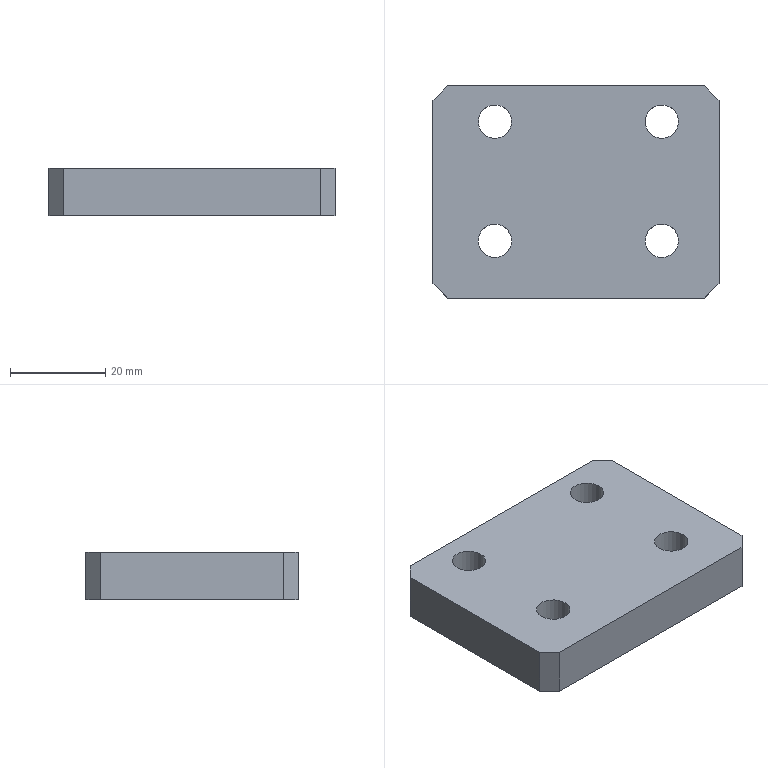Part | NX | features BREP 1 | 1 solid | 14 faces | box 60 x 44.5 x 10 mm | volume 24981 mm3 | plane 10 | cylinder 4 | commonest cylinder face diameters 7 x4
STEP:
#1=CARTESIAN_POINT('',(30.,-19.25,0.));
#2=VERTEX_POINT('',#1);
#3=CARTESIAN_POINT('',(30.,19.25,0.));
#4=VERTEX_POINT('',#3);
#5=CARTESIAN_POINT('',(30.,22.25,0.));
#6=DIRECTION('',(0.,1.,0.));
#7=VECTOR('',#6,1000.);
#8=LINE('',#5,#7);
#9=EDGE_CURVE('',#2,#4,#8,.T.);
#10=ORIENTED_EDGE('',*,*,#9,.T.);
#11=CARTESIAN_POINT('',(30.,19.25,10.));
#12=VERTEX_POINT('',#11);
#13=CARTESIAN_POINT('',(30.,19.25,10.));
#14=DIRECTION('',(0.,0.,1.));
#15=VECTOR('',#14,1000.);
#16=LINE('',#13,#15);
#17=EDGE_CURVE('',#4,#12,#16,.T.);
#18=ORIENTED_EDGE('',*,*,#17,.T.);
#19=CARTESIAN_POINT('',(30.,-19.25,10.));
#20=VERTEX_POINT('',#19);
#21=CARTESIAN_POINT('',(30.,22.25,10.));
#22=DIRECTION('',(0.,1.,0.));
#23=VECTOR('',#22,1000.);
#24=LINE('',#21,#23);
#25=EDGE_CURVE('',#20,#12,#24,.T.);
#26=ORIENTED_EDGE('',*,*,#25,.F.);
#27=CARTESIAN_POINT('',(30.,-19.25,10.));
#28=DIRECTION('',(0.,0.,-1.));
#29=VECTOR('',#28,1000.);
#30=LINE('',#27,#29);
#31=EDGE_CURVE('',#20,#2,#30,.T.);
#32=ORIENTED_EDGE('',*,*,#31,.T.);
#33=EDGE_LOOP('',(#10,#18,#26,#32));
#34=FACE_BOUND('',#33,.T.);
#35=CARTESIAN_POINT('',(30.,22.25,10.));
#36=DIRECTION('',(-1.,0.,0.));
#37=DIRECTION('',(0.,1.,0.));
#38=AXIS2_PLACEMENT_3D('',#35,#36,#37);
#39=PLANE('',#38);
#40=ADVANCED_FACE('',(#34),#39,.F.);
#41=CARTESIAN_POINT('',(27.,22.25,10.));
#42=VERTEX_POINT('',#41);
#43=CARTESIAN_POINT('',(-27.,22.25,10.));
#44=VERTEX_POINT('',#43);
#45=CARTESIAN_POINT('',(-30.,22.25,10.));
#46=DIRECTION('',(-1.,0.,0.));
#47=VECTOR('',#46,1000.);
#48=LINE('',#45,#47);
#49=EDGE_CURVE('',#42,#44,#48,.T.);
#50=ORIENTED_EDGE('',*,*,#49,.F.);
#51=CARTESIAN_POINT('',(27.,22.25,0.));
#52=VERTEX_POINT('',#51);
#53=CARTESIAN_POINT('',(27.,22.25,10.));
#54=DIRECTION('',(0.,0.,-1.));
#55=VECTOR('',#54,1000.);
#56=LINE('',#53,#55);
#57=EDGE_CURVE('',#42,#52,#56,.T.);
#58=ORIENTED_EDGE('',*,*,#57,.T.);
#59=CARTESIAN_POINT('',(-27.,22.25,0.));
#60=VERTEX_POINT('',#59);
#61=CARTESIAN_POINT('',(-30.,22.25,0.));
#62=DIRECTION('',(-1.,0.,0.));
#63=VECTOR('',#62,1000.);
#64=LINE('',#61,#63);
#65=EDGE_CURVE('',#52,#60,#64,.T.);
#66=ORIENTED_EDGE('',*,*,#65,.T.);
#67=CARTESIAN_POINT('',(-27.,22.25,10.));
#68=DIRECTION('',(0.,0.,1.));
#69=VECTOR('',#68,1000.);
#70=LINE('',#67,#69);
#71=EDGE_CURVE('',#60,#44,#70,.T.);
#72=ORIENTED_EDGE('',*,*,#71,.T.);
#73=EDGE_LOOP('',(#50,#58,#66,#72));
#74=FACE_BOUND('',#73,.T.);
#75=CARTESIAN_POINT('',(-30.,22.25,10.));
#76=DIRECTION('',(0.,-1.,0.));
#77=DIRECTION('',(0.,0.,1.));
#78=AXIS2_PLACEMENT_3D('',#75,#76,#77);
#79=PLANE('',#78);
#80=ADVANCED_FACE('',(#74),#79,.F.);
#81=CARTESIAN_POINT('',(-30.,19.25,10.));
#82=VERTEX_POINT('',#81);
#83=CARTESIAN_POINT('',(-30.,-19.25,10.));
#84=VERTEX_POINT('',#83);
#85=CARTESIAN_POINT('',(-30.,22.25,10.));
#86=DIRECTION('',(0.,-1.,0.));
#87=VECTOR('',#86,1000.);
#88=LINE('',#85,#87);
#89=EDGE_CURVE('',#82,#84,#88,.T.);
#90=ORIENTED_EDGE('',*,*,#89,.F.);
#91=CARTESIAN_POINT('',(-30.,19.25,0.));
#92=VERTEX_POINT('',#91);
#93=CARTESIAN_POINT('',(-30.,19.25,10.));
#94=DIRECTION('',(0.,0.,-1.));
#95=VECTOR('',#94,1000.);
#96=LINE('',#93,#95);
#97=EDGE_CURVE('',#82,#92,#96,.T.);
#98=ORIENTED_EDGE('',*,*,#97,.T.);
#99=CARTESIAN_POINT('',(-30.,-19.25,0.));
#100=VERTEX_POINT('',#99);
#101=CARTESIAN_POINT('',(-30.,22.25,0.));
#102=DIRECTION('',(0.,-1.,0.));
#103=VECTOR('',#102,1000.);
#104=LINE('',#101,#103);
#105=EDGE_CURVE('',#92,#100,#104,.T.);
#106=ORIENTED_EDGE('',*,*,#105,.T.);
#107=CARTESIAN_POINT('',(-30.,-19.25,10.));
#108=DIRECTION('',(0.,0.,1.));
#109=VECTOR('',#108,1000.);
#110=LINE('',#107,#109);
#111=EDGE_CURVE('',#100,#84,#110,.T.);
#112=ORIENTED_EDGE('',*,*,#111,.T.);
#113=EDGE_LOOP('',(#90,#98,#106,#112));
#114=FACE_BOUND('',#113,.T.);
#115=CARTESIAN_POINT('',(-30.,22.25,10.));
#116=DIRECTION('',(1.,0.,0.));
#117=DIRECTION('',(0.,-1.,0.));
#118=AXIS2_PLACEMENT_3D('',#115,#116,#117);
#119=PLANE('',#118);
#120=ADVANCED_FACE('',(#114),#119,.F.);
#121=CARTESIAN_POINT('',(-27.,-22.25,0.));
#122=VERTEX_POINT('',#121);
#123=CARTESIAN_POINT('',(27.,-22.25,0.));
#124=VERTEX_POINT('',#123);
#125=CARTESIAN_POINT('',(-30.,-22.25,0.));
#126=DIRECTION('',(1.,0.,0.));
#127=VECTOR('',#126,1000.);
#128=LINE('',#125,#127);
#129=EDGE_CURVE('',#122,#124,#128,.T.);
#130=ORIENTED_EDGE('',*,*,#129,.T.);
#131=CARTESIAN_POINT('',(27.,-22.25,10.));
#132=VERTEX_POINT('',#131);
#133=CARTESIAN_POINT('',(27.,-22.25,10.));
#134=DIRECTION('',(0.,0.,1.));
#135=VECTOR('',#134,1000.);
#136=LINE('',#133,#135);
#137=EDGE_CURVE('',#124,#132,#136,.T.);
#138=ORIENTED_EDGE('',*,*,#137,.T.);
#139=CARTESIAN_POINT('',(-27.,-22.25,10.));
#140=VERTEX_POINT('',#139);
#141=CARTESIAN_POINT('',(-30.,-22.25,10.));
#142=DIRECTION('',(1.,0.,0.));
#143=VECTOR('',#142,1000.);
#144=LINE('',#141,#143);
#145=EDGE_CURVE('',#140,#132,#144,.T.);
#146=ORIENTED_EDGE('',*,*,#145,.F.);
#147=CARTESIAN_POINT('',(-27.,-22.25,10.));
#148=DIRECTION('',(0.,0.,-1.));
#149=VECTOR('',#148,1000.);
#150=LINE('',#147,#149);
#151=EDGE_CURVE('',#140,#122,#150,.T.);
#152=ORIENTED_EDGE('',*,*,#151,.T.);
#153=EDGE_LOOP('',(#130,#138,#146,#152));
#154=FACE_BOUND('',#153,.T.);
#155=CARTESIAN_POINT('',(-30.,-22.25,10.));
#156=DIRECTION('',(0.,1.,0.));
#157=DIRECTION('',(0.,0.,-1.));
#158=AXIS2_PLACEMENT_3D('',#155,#156,#157);
#159=PLANE('',#158);
#160=ADVANCED_FACE('',(#154),#159,.F.);
#161=CARTESIAN_POINT('',(-20.5,-10.25,10.));
#162=VERTEX_POINT('',#161);
#163=CARTESIAN_POINT('',(-17.,-10.25,10.));
#164=DIRECTION('',(0.,0.,-1.));
#165=DIRECTION('',(-1.,0.,0.));
#166=AXIS2_PLACEMENT_3D('',#163,#164,#165);
#167=CIRCLE('',#166,3.5);
#168=EDGE_CURVE('',#162,#162,#167,.T.);
#169=ORIENTED_EDGE('',*,*,#168,.T.);
#170=EDGE_LOOP('',(#169));
#171=FACE_BOUND('',#170,.T.);
#172=CARTESIAN_POINT('',(-20.5,14.75,10.));
#173=VERTEX_POINT('',#172);
#174=CARTESIAN_POINT('',(-17.,14.75,10.));
#175=DIRECTION('',(0.,0.,-1.));
#176=DIRECTION('',(-1.,0.,0.));
#177=AXIS2_PLACEMENT_3D('',#174,#175,#176);
#178=CIRCLE('',#177,3.5);
#179=EDGE_CURVE('',#173,#173,#178,.T.);
#180=ORIENTED_EDGE('',*,*,#179,.T.);
#181=EDGE_LOOP('',(#180));
#182=FACE_BOUND('',#181,.T.);
#183=CARTESIAN_POINT('',(14.5,-10.25,10.));
#184=VERTEX_POINT('',#183);
#185=CARTESIAN_POINT('',(18.,-10.25,10.));
#186=DIRECTION('',(0.,0.,-1.));
#187=DIRECTION('',(-1.,0.,0.));
#188=AXIS2_PLACEMENT_3D('',#185,#186,#187);
#189=CIRCLE('',#188,3.5);
#190=EDGE_CURVE('',#184,#184,#189,.T.);
#191=ORIENTED_EDGE('',*,*,#190,.T.);
#192=EDGE_LOOP('',(#191));
#193=FACE_BOUND('',#192,.T.);
#194=CARTESIAN_POINT('',(14.5,14.75,10.));
#195=VERTEX_POINT('',#194);
#196=CARTESIAN_POINT('',(18.,14.75,10.));
#197=DIRECTION('',(0.,0.,-1.));
#198=DIRECTION('',(-1.,0.,0.));
#199=AXIS2_PLACEMENT_3D('',#196,#197,#198);
#200=CIRCLE('',#199,3.5);
#201=EDGE_CURVE('',#195,#195,#200,.T.);
#202=ORIENTED_EDGE('',*,*,#201,.T.);
#203=EDGE_LOOP('',(#202));
#204=FACE_BOUND('',#203,.T.);
#205=ORIENTED_EDGE('',*,*,#25,.T.);
#206=CARTESIAN_POINT('',(24.625,24.625,10.));
#207=DIRECTION('',(-0.7071,0.7071,0.));
#208=VECTOR('',#207,1000.);
#209=LINE('',#206,#208);
#210=EDGE_CURVE('',#12,#42,#209,.T.);
#211=ORIENTED_EDGE('',*,*,#210,.T.);
#212=ORIENTED_EDGE('',*,*,#49,.T.);
#213=CARTESIAN_POINT('',(-24.625,24.625,10.));
#214=DIRECTION('',(-0.7071,-0.7071,0.));
#215=VECTOR('',#214,1000.);
#216=LINE('',#213,#215);
#217=EDGE_CURVE('',#44,#82,#216,.T.);
#218=ORIENTED_EDGE('',*,*,#217,.T.);
#219=ORIENTED_EDGE('',*,*,#89,.T.);
#220=CARTESIAN_POINT('',(-24.625,-24.625,10.));
#221=DIRECTION('',(0.7071,-0.7071,0.));
#222=VECTOR('',#221,1000.);
#223=LINE('',#220,#222);
#224=EDGE_CURVE('',#84,#140,#223,.T.);
#225=ORIENTED_EDGE('',*,*,#224,.T.);
#226=ORIENTED_EDGE('',*,*,#145,.T.);
#227=CARTESIAN_POINT('',(24.625,-24.625,10.));
#228=DIRECTION('',(0.7071,0.7071,0.));
#229=VECTOR('',#228,1000.);
#230=LINE('',#227,#229);
#231=EDGE_CURVE('',#132,#20,#230,.T.);
#232=ORIENTED_EDGE('',*,*,#231,.T.);
#233=EDGE_LOOP('',(#205,#211,#212,#218,#219,#225,#226,#232));
#234=FACE_BOUND('',#233,.T.);
#235=CARTESIAN_POINT('',(0.,0.,10.));
#236=DIRECTION('',(0.,0.,1.));
#237=DIRECTION('',(-1.,0.,0.));
#238=AXIS2_PLACEMENT_3D('',#235,#236,#237);
#239=PLANE('',#238);
#240=ADVANCED_FACE('',(#171,#182,#193,#204,#234),#239,.T.);
#241=CARTESIAN_POINT('',(-20.5,-10.25,0.));
#242=VERTEX_POINT('',#241);
#243=CARTESIAN_POINT('',(-17.,-10.25,0.));
#244=DIRECTION('',(0.,0.,-1.));
#245=DIRECTION('',(-1.,0.,0.));
#246=AXIS2_PLACEMENT_3D('',#243,#244,#245);
#247=CIRCLE('',#246,3.5);
#248=EDGE_CURVE('',#242,#242,#247,.T.);
#249=ORIENTED_EDGE('',*,*,#248,.F.);
#250=EDGE_LOOP('',(#249));
#251=FACE_BOUND('',#250,.T.);
#252=CARTESIAN_POINT('',(-20.5,14.75,0.));
#253=VERTEX_POINT('',#252);
#254=CARTESIAN_POINT('',(-17.,14.75,0.));
#255=DIRECTION('',(0.,0.,-1.));
#256=DIRECTION('',(-1.,0.,0.));
#257=AXIS2_PLACEMENT_3D('',#254,#255,#256);
#258=CIRCLE('',#257,3.5);
#259=EDGE_CURVE('',#253,#253,#258,.T.);
#260=ORIENTED_EDGE('',*,*,#259,.F.);
#261=EDGE_LOOP('',(#260));
#262=FACE_BOUND('',#261,.T.);
#263=CARTESIAN_POINT('',(14.5,-10.25,0.));
#264=VERTEX_POINT('',#263);
#265=CARTESIAN_POINT('',(18.,-10.25,0.));
#266=DIRECTION('',(0.,0.,-1.));
#267=DIRECTION('',(-1.,0.,0.));
#268=AXIS2_PLACEMENT_3D('',#265,#266,#267);
#269=CIRCLE('',#268,3.5);
#270=EDGE_CURVE('',#264,#264,#269,.T.);
#271=ORIENTED_EDGE('',*,*,#270,.F.);
#272=EDGE_LOOP('',(#271));
#273=FACE_BOUND('',#272,.T.);
#274=CARTESIAN_POINT('',(14.5,14.75,0.));
#275=VERTEX_POINT('',#274);
#276=CARTESIAN_POINT('',(18.,14.75,0.));
#277=DIRECTION('',(0.,0.,-1.));
#278=DIRECTION('',(-1.,0.,0.));
#279=AXIS2_PLACEMENT_3D('',#276,#277,#278);
#280=CIRCLE('',#279,3.5);
#281=EDGE_CURVE('',#275,#275,#280,.T.);
#282=ORIENTED_EDGE('',*,*,#281,.F.);
#283=EDGE_LOOP('',(#282));
#284=FACE_BOUND('',#283,.T.);
#285=ORIENTED_EDGE('',*,*,#65,.F.);
#286=CARTESIAN_POINT('',(27.,22.25,0.));
#287=DIRECTION('',(0.7071,-0.7071,0.));
#288=VECTOR('',#287,1000.);
#289=LINE('',#286,#288);
#290=EDGE_CURVE('',#52,#4,#289,.T.);
#291=ORIENTED_EDGE('',*,*,#290,.T.);
#292=ORIENTED_EDGE('',*,*,#9,.F.);
#293=CARTESIAN_POINT('',(30.,-19.25,0.));
#294=DIRECTION('',(-0.7071,-0.7071,0.));
#295=VECTOR('',#294,1000.);
#296=LINE('',#293,#295);
#297=EDGE_CURVE('',#2,#124,#296,.T.);
#298=ORIENTED_EDGE('',*,*,#297,.T.);
#299=ORIENTED_EDGE('',*,*,#129,.F.);
#300=CARTESIAN_POINT('',(-27.,-22.25,0.));
#301=DIRECTION('',(-0.7071,0.7071,0.));
#302=VECTOR('',#301,1000.);
#303=LINE('',#300,#302);
#304=EDGE_CURVE('',#122,#100,#303,.T.);
#305=ORIENTED_EDGE('',*,*,#304,.T.);
#306=ORIENTED_EDGE('',*,*,#105,.F.);
#307=CARTESIAN_POINT('',(-30.,19.25,0.));
#308=DIRECTION('',(0.7071,0.7071,0.));
#309=VECTOR('',#308,1000.);
#310=LINE('',#307,#309);
#311=EDGE_CURVE('',#92,#60,#310,.T.);
#312=ORIENTED_EDGE('',*,*,#311,.T.);
#313=EDGE_LOOP('',(#285,#291,#292,#298,#299,#305,#306,#312));
#314=FACE_BOUND('',#313,.T.);
#315=CARTESIAN_POINT('',(0.,0.,0.));
#316=DIRECTION('',(0.,0.,1.));
#317=DIRECTION('',(-1.,0.,0.));
#318=AXIS2_PLACEMENT_3D('',#315,#316,#317);
#319=PLANE('',#318);
#320=ADVANCED_FACE('',(#251,#262,#273,#284,#314),#319,.F.);
#321=ORIENTED_EDGE('',*,*,#201,.F.);
#322=EDGE_LOOP('',(#321));
#323=FACE_BOUND('',#322,.T.);
#324=ORIENTED_EDGE('',*,*,#281,.T.);
#325=EDGE_LOOP('',(#324));
#326=FACE_BOUND('',#325,.T.);
#327=CARTESIAN_POINT('',(18.,14.75,0.));
#328=DIRECTION('',(0.,0.,-1.));
#329=DIRECTION('',(1.,0.,0.));
#330=AXIS2_PLACEMENT_3D('',#327,#328,#329);
#331=CYLINDRICAL_SURFACE('',#330,3.5);
#332=ADVANCED_FACE('',(#323,#326),#331,.F.);
#333=ORIENTED_EDGE('',*,*,#190,.F.);
#334=EDGE_LOOP('',(#333));
#335=FACE_BOUND('',#334,.T.);
#336=ORIENTED_EDGE('',*,*,#270,.T.);
#337=EDGE_LOOP('',(#336));
#338=FACE_BOUND('',#337,.T.);
#339=CARTESIAN_POINT('',(18.,-10.25,0.));
#340=DIRECTION('',(0.,0.,-1.));
#341=DIRECTION('',(1.,0.,0.));
#342=AXIS2_PLACEMENT_3D('',#339,#340,#341);
#343=CYLINDRICAL_SURFACE('',#342,3.5);
#344=ADVANCED_FACE('',(#335,#338),#343,.F.);
#345=ORIENTED_EDGE('',*,*,#179,.F.);
#346=EDGE_LOOP('',(#345));
#347=FACE_BOUND('',#346,.T.);
#348=ORIENTED_EDGE('',*,*,#259,.T.);
#349=EDGE_LOOP('',(#348));
#350=FACE_BOUND('',#349,.T.);
#351=CARTESIAN_POINT('',(-17.,14.75,0.));
#352=DIRECTION('',(0.,0.,-1.));
#353=DIRECTION('',(1.,0.,0.));
#354=AXIS2_PLACEMENT_3D('',#351,#352,#353);
#355=CYLINDRICAL_SURFACE('',#354,3.5);
#356=ADVANCED_FACE('',(#347,#350),#355,.F.);
#357=ORIENTED_EDGE('',*,*,#168,.F.);
#358=EDGE_LOOP('',(#357));
#359=FACE_BOUND('',#358,.T.);
#360=ORIENTED_EDGE('',*,*,#248,.T.);
#361=EDGE_LOOP('',(#360));
#362=FACE_BOUND('',#361,.T.);
#363=CARTESIAN_POINT('',(-17.,-10.25,0.));
#364=DIRECTION('',(0.,0.,-1.));
#365=DIRECTION('',(1.,0.,0.));
#366=AXIS2_PLACEMENT_3D('',#363,#364,#365);
#367=CYLINDRICAL_SURFACE('',#366,3.5);
#368=ADVANCED_FACE('',(#359,#362),#367,.F.);
#369=ORIENTED_EDGE('',*,*,#210,.F.);
#370=ORIENTED_EDGE('',*,*,#17,.F.);
#371=ORIENTED_EDGE('',*,*,#290,.F.);
#372=ORIENTED_EDGE('',*,*,#57,.F.);
#373=EDGE_LOOP('',(#369,#370,#371,#372));
#374=FACE_BOUND('',#373,.T.);
#375=CARTESIAN_POINT('',(27.,22.25,10.));
#376=DIRECTION('',(-0.7071,-0.7071,0.));
#377=DIRECTION('',(0.,0.,1.));
#378=AXIS2_PLACEMENT_3D('',#375,#376,#377);
#379=PLANE('',#378);
#380=ADVANCED_FACE('',(#374),#379,.F.);
#381=ORIENTED_EDGE('',*,*,#231,.F.);
#382=ORIENTED_EDGE('',*,*,#137,.F.);
#383=ORIENTED_EDGE('',*,*,#297,.F.);
#384=ORIENTED_EDGE('',*,*,#31,.F.);
#385=EDGE_LOOP('',(#381,#382,#383,#384));
#386=FACE_BOUND('',#385,.T.);
#387=CARTESIAN_POINT('',(30.,-19.25,10.));
#388=DIRECTION('',(-0.7071,0.7071,0.));
#389=DIRECTION('',(0.,0.,1.));
#390=AXIS2_PLACEMENT_3D('',#387,#388,#389);
#391=PLANE('',#390);
#392=ADVANCED_FACE('',(#386),#391,.F.);
#393=ORIENTED_EDGE('',*,*,#217,.F.);
#394=ORIENTED_EDGE('',*,*,#71,.F.);
#395=ORIENTED_EDGE('',*,*,#311,.F.);
#396=ORIENTED_EDGE('',*,*,#97,.F.);
#397=EDGE_LOOP('',(#393,#394,#395,#396));
#398=FACE_BOUND('',#397,.T.);
#399=CARTESIAN_POINT('',(-30.,19.25,10.));
#400=DIRECTION('',(0.7071,-0.7071,0.));
#401=DIRECTION('',(0.,0.,1.));
#402=AXIS2_PLACEMENT_3D('',#399,#400,#401);
#403=PLANE('',#402);
#404=ADVANCED_FACE('',(#398),#403,.F.);
#405=ORIENTED_EDGE('',*,*,#224,.F.);
#406=ORIENTED_EDGE('',*,*,#111,.F.);
#407=ORIENTED_EDGE('',*,*,#304,.F.);
#408=ORIENTED_EDGE('',*,*,#151,.F.);
#409=EDGE_LOOP('',(#405,#406,#407,#408));
#410=FACE_BOUND('',#409,.T.);
#411=CARTESIAN_POINT('',(-27.,-22.25,10.));
#412=DIRECTION('',(0.7071,0.7071,0.));
#413=DIRECTION('',(0.,0.,1.));
#414=AXIS2_PLACEMENT_3D('',#411,#412,#413);
#415=PLANE('',#414);
#416=ADVANCED_FACE('',(#410),#415,.F.);
#417=CLOSED_SHELL('',(#40,#80,#120,#160,#240,#320,#332,#344,#356,#368,#380,#392,#404,#416));
#418=MANIFOLD_SOLID_BREP('',#417);
#419=(LENGTH_UNIT()NAMED_UNIT(*)SI_UNIT(.MILLI.,.METRE.));
#420=UNCERTAINTY_MEASURE_WITH_UNIT(LENGTH_MEASURE(0.00001),#419,'','');
#421=(NAMED_UNIT(*)PLANE_ANGLE_UNIT()SI_UNIT($,.RADIAN.));
#422=(NAMED_UNIT(*)SI_UNIT($,.STERADIAN.)SOLID_ANGLE_UNIT());
#423=(GEOMETRIC_REPRESENTATION_CONTEXT(3)GLOBAL_UNCERTAINTY_ASSIGNED_CONTEXT((#420))GLOBAL_UNIT_ASSIGNED_CONTEXT((#419,#421,#422))REPRESENTATION_CONTEXT('',''));
#424=ADVANCED_BREP_SHAPE_REPRESENTATION('',(#418),#423);